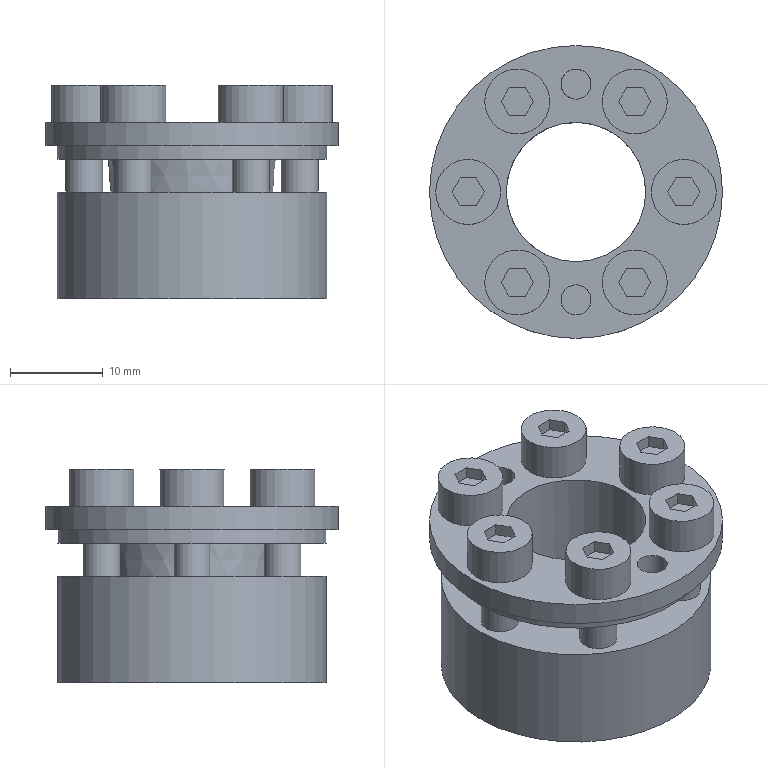Part | NX | features 5003_003_MLMB15 2 | 1 solid | 91 faces | box 31.5 x 31.5 x 23 mm | volume 8591 mm3 | plane 64 | cylinder 24 | cone 2 | spline 1 | commonest cylinder face diameters 3.242 x8 4 x6 7 x6 29 x2 15 x1 31.5 x1